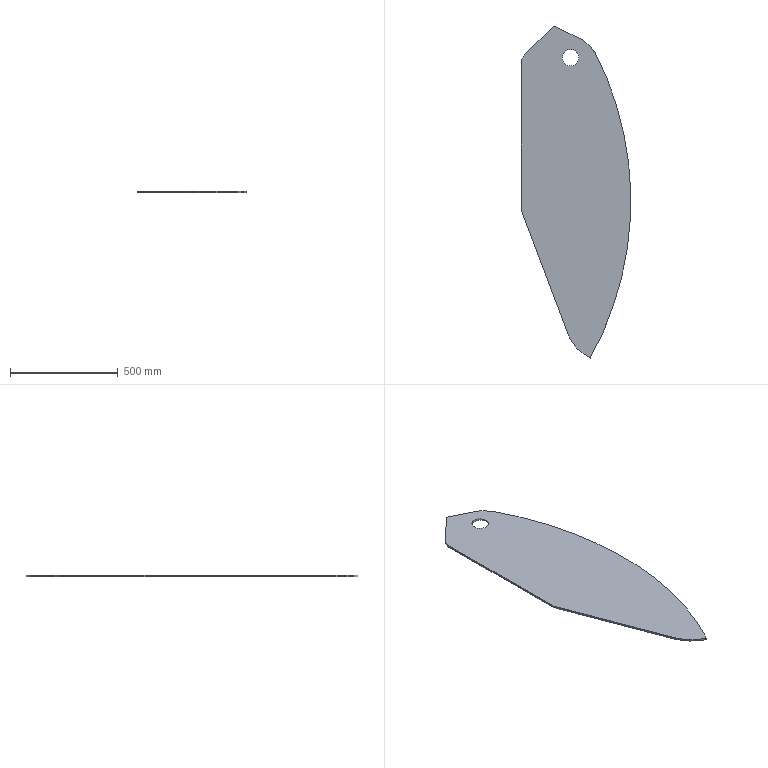Part | SolidWorks | features Extrusion 1 | 1 solid | 13 faces | box 508 x 1540 x 8 mm | volume 4517145 mm3 | plane 7 | cylinder 6 | commonest cylinder face diameters 76.2 x2 101.6 x1 279.4 x1 406.4 x1 3016 x1
STEP:
#1=CARTESIAN_POINT('',(1190.625,663.575,4.));
#2=VERTEX_POINT('',#1);
#3=CARTESIAN_POINT('',(1266.825,663.575,4.));
#4=VERTEX_POINT('',#3);
#5=CARTESIAN_POINT('',(1228.725,663.575,4.));
#6=DIRECTION('',(0.,0.,1.));
#7=DIRECTION('',(1.,0.,0.));
#8=AXIS2_PLACEMENT_3D('',#5,#6,#7);
#9=CIRCLE('',#8,38.1);
#10=EDGE_CURVE('',#2,#4,#9,.T.);
#11=ORIENTED_EDGE('',*,*,#10,.T.);
#12=CARTESIAN_POINT('',(1266.825,663.575,-4.));
#13=VERTEX_POINT('',#12);
#14=CARTESIAN_POINT('',(1266.825,663.575,4.));
#15=DIRECTION('',(0.,0.,-1.));
#16=VECTOR('',#15,1000.);
#17=LINE('',#14,#16);
#18=EDGE_CURVE('',#4,#13,#17,.T.);
#19=ORIENTED_EDGE('',*,*,#18,.T.);
#20=CARTESIAN_POINT('',(1190.625,663.575,-4.));
#21=VERTEX_POINT('',#20);
#22=CARTESIAN_POINT('',(1228.725,663.575,-4.));
#23=DIRECTION('',(0.,0.,1.));
#24=DIRECTION('',(1.,0.,0.));
#25=AXIS2_PLACEMENT_3D('',#22,#23,#24);
#26=CIRCLE('',#25,38.1);
#27=EDGE_CURVE('',#21,#13,#26,.T.);
#28=ORIENTED_EDGE('',*,*,#27,.F.);
#29=CARTESIAN_POINT('',(1190.625,663.575,4.));
#30=DIRECTION('',(0.,0.,-1.));
#31=VECTOR('',#30,1000.);
#32=LINE('',#29,#31);
#33=EDGE_CURVE('',#2,#21,#32,.T.);
#34=ORIENTED_EDGE('',*,*,#33,.F.);
#35=EDGE_LOOP('',(#11,#19,#28,#34));
#36=FACE_OUTER_BOUND('',#35,.T.);
#37=CARTESIAN_POINT('',(1228.725,663.575,4.));
#38=DIRECTION('',(0.,0.,-1.));
#39=DIRECTION('',(-1.,0.,0.));
#40=AXIS2_PLACEMENT_3D('',#37,#38,#39);
#41=CYLINDRICAL_SURFACE('',#40,38.1);
#42=ADVANCED_FACE('',(#36),#41,.F.);
#43=CARTESIAN_POINT('',(1015.696,677.95,4.));
#44=VERTEX_POINT('',#43);
#45=CARTESIAN_POINT('',(1000.125,641.35,4.));
#46=VERTEX_POINT('',#45);
#47=CARTESIAN_POINT('',(1050.925,641.35,4.));
#48=DIRECTION('',(0.,0.,1.));
#49=DIRECTION('',(1.,0.,0.));
#50=AXIS2_PLACEMENT_3D('',#47,#48,#49);
#51=CIRCLE('',#50,50.8);
#52=EDGE_CURVE('',#44,#46,#51,.T.);
#53=ORIENTED_EDGE('',*,*,#52,.T.);
#54=CARTESIAN_POINT('',(1000.125,-45.063,4.));
#55=VERTEX_POINT('',#54);
#56=CARTESIAN_POINT('',(1000.125,641.35,4.));
#57=DIRECTION('',(0.,-1.,0.));
#58=VECTOR('',#57,1000.);
#59=LINE('',#56,#58);
#60=EDGE_CURVE('',#46,#55,#59,.T.);
#61=ORIENTED_EDGE('',*,*,#60,.T.);
#62=CARTESIAN_POINT('',(1215.934,-617.114,4.));
#63=VERTEX_POINT('',#62);
#64=CARTESIAN_POINT('',(1000.125,-45.063,4.));
#65=DIRECTION('',(0.353,-0.9356,0.));
#66=VECTOR('',#65,1000.);
#67=LINE('',#64,#66);
#68=EDGE_CURVE('',#55,#63,#67,.T.);
#69=ORIENTED_EDGE('',*,*,#68,.T.);
#70=CARTESIAN_POINT('',(1319.975,-729.456,4.));
#71=VERTEX_POINT('',#70);
#72=CARTESIAN_POINT('',(1406.055,-545.39,4.));
#73=DIRECTION('',(0.,0.,1.));
#74=DIRECTION('',(1.,0.,0.));
#75=AXIS2_PLACEMENT_3D('',#72,#73,#74);
#76=CIRCLE('',#75,203.2);
#77=EDGE_CURVE('',#63,#71,#76,.T.);
#78=ORIENTED_EDGE('',*,*,#77,.T.);
#79=CARTESIAN_POINT('',(1339.914,692.15,4.));
#80=VERTEX_POINT('',#79);
#81=CARTESIAN_POINT('',(0.,0.,4.));
#82=DIRECTION('',(0.,0.,1.));
#83=DIRECTION('',(1.,0.,0.));
#84=AXIS2_PLACEMENT_3D('',#81,#82,#83);
#85=CIRCLE('',#84,1508.125);
#86=EDGE_CURVE('',#71,#80,#85,.T.);
#87=ORIENTED_EDGE('',*,*,#86,.T.);
#88=CARTESIAN_POINT('',(1336.871,690.572,4.));
#89=VERTEX_POINT('',#88);
#90=CARTESIAN_POINT('',(1339.914,692.15,4.));
#91=DIRECTION('',(-0.8878,-0.4603,0.));
#92=VECTOR('',#91,1000.);
#93=LINE('',#90,#92);
#94=EDGE_CURVE('',#80,#89,#93,.T.);
#95=ORIENTED_EDGE('',*,*,#94,.T.);
#96=CARTESIAN_POINT('',(1273.824,751.96,4.));
#97=VERTEX_POINT('',#96);
#98=CARTESIAN_POINT('',(1212.85,626.269,4.));
#99=DIRECTION('',(0.,0.,1.));
#100=DIRECTION('',(1.,0.,0.));
#101=AXIS2_PLACEMENT_3D('',#98,#99,#100);
#102=CIRCLE('',#101,139.7);
#103=EDGE_CURVE('',#89,#97,#102,.T.);
#104=ORIENTED_EDGE('',*,*,#103,.T.);
#105=CARTESIAN_POINT('',(1153.319,810.419,4.));
#106=VERTEX_POINT('',#105);
#107=CARTESIAN_POINT('',(1153.319,810.419,4.));
#108=DIRECTION('',(-0.8997,0.4365,0.));
#109=VECTOR('',#108,1000.);
#110=LINE('',#107,#109);
#111=EDGE_CURVE('',#97,#106,#110,.T.);
#112=ORIENTED_EDGE('',*,*,#111,.T.);
#113=CARTESIAN_POINT('',(1153.319,810.419,4.));
#114=DIRECTION('',(-0.7205,-0.6935,0.));
#115=VECTOR('',#114,1000.);
#116=LINE('',#113,#115);
#117=EDGE_CURVE('',#106,#44,#116,.T.);
#118=ORIENTED_EDGE('',*,*,#117,.T.);
#119=EDGE_LOOP('',(#53,#61,#69,#78,#87,#95,#104,#112,#118));
#120=FACE_OUTER_BOUND('',#119,.T.);
#121=ORIENTED_EDGE('',*,*,#10,.F.);
#122=CARTESIAN_POINT('',(1228.725,663.575,4.));
#123=DIRECTION('',(0.,0.,1.));
#124=DIRECTION('',(1.,0.,0.));
#125=AXIS2_PLACEMENT_3D('',#122,#123,#124);
#126=CIRCLE('',#125,38.1);
#127=EDGE_CURVE('',#4,#2,#126,.T.);
#128=ORIENTED_EDGE('',*,*,#127,.F.);
#129=EDGE_LOOP('',(#121,#128));
#130=FACE_BOUND('',#129,.T.);
#131=CARTESIAN_POINT('',(1050.925,641.35,4.));
#132=DIRECTION('',(0.,0.,1.));
#133=DIRECTION('',(1.,0.,0.));
#134=AXIS2_PLACEMENT_3D('',#131,#132,#133);
#135=PLANE('',#134);
#136=ADVANCED_FACE('',(#120,#130),#135,.T.);
#137=CARTESIAN_POINT('',(1015.696,677.95,-4.));
#138=VERTEX_POINT('',#137);
#139=CARTESIAN_POINT('',(1000.125,641.35,-4.));
#140=VERTEX_POINT('',#139);
#141=CARTESIAN_POINT('',(1050.925,641.35,-4.));
#142=DIRECTION('',(0.,0.,1.));
#143=DIRECTION('',(1.,0.,0.));
#144=AXIS2_PLACEMENT_3D('',#141,#142,#143);
#145=CIRCLE('',#144,50.8);
#146=EDGE_CURVE('',#138,#140,#145,.T.);
#147=ORIENTED_EDGE('',*,*,#146,.F.);
#148=CARTESIAN_POINT('',(1153.319,810.419,-4.));
#149=VERTEX_POINT('',#148);
#150=CARTESIAN_POINT('',(1153.319,810.419,-4.));
#151=DIRECTION('',(-0.7205,-0.6935,0.));
#152=VECTOR('',#151,1000.);
#153=LINE('',#150,#152);
#154=EDGE_CURVE('',#149,#138,#153,.T.);
#155=ORIENTED_EDGE('',*,*,#154,.F.);
#156=CARTESIAN_POINT('',(1273.824,751.96,-4.));
#157=VERTEX_POINT('',#156);
#158=CARTESIAN_POINT('',(1153.319,810.419,-4.));
#159=DIRECTION('',(-0.8997,0.4365,0.));
#160=VECTOR('',#159,1000.);
#161=LINE('',#158,#160);
#162=EDGE_CURVE('',#157,#149,#161,.T.);
#163=ORIENTED_EDGE('',*,*,#162,.F.);
#164=CARTESIAN_POINT('',(1336.871,690.572,-4.));
#165=VERTEX_POINT('',#164);
#166=CARTESIAN_POINT('',(1212.85,626.269,-4.));
#167=DIRECTION('',(0.,0.,1.));
#168=DIRECTION('',(1.,0.,0.));
#169=AXIS2_PLACEMENT_3D('',#166,#167,#168);
#170=CIRCLE('',#169,139.7);
#171=EDGE_CURVE('',#165,#157,#170,.T.);
#172=ORIENTED_EDGE('',*,*,#171,.F.);
#173=CARTESIAN_POINT('',(1339.914,692.15,-4.));
#174=VERTEX_POINT('',#173);
#175=CARTESIAN_POINT('',(1339.914,692.15,-4.));
#176=DIRECTION('',(-0.8878,-0.4603,0.));
#177=VECTOR('',#176,1000.);
#178=LINE('',#175,#177);
#179=EDGE_CURVE('',#174,#165,#178,.T.);
#180=ORIENTED_EDGE('',*,*,#179,.F.);
#181=CARTESIAN_POINT('',(1319.975,-729.456,-4.));
#182=VERTEX_POINT('',#181);
#183=CARTESIAN_POINT('',(0.,0.,-4.));
#184=DIRECTION('',(0.,0.,1.));
#185=DIRECTION('',(1.,0.,0.));
#186=AXIS2_PLACEMENT_3D('',#183,#184,#185);
#187=CIRCLE('',#186,1508.125);
#188=EDGE_CURVE('',#182,#174,#187,.T.);
#189=ORIENTED_EDGE('',*,*,#188,.F.);
#190=CARTESIAN_POINT('',(1215.934,-617.114,-4.));
#191=VERTEX_POINT('',#190);
#192=CARTESIAN_POINT('',(1406.055,-545.39,-4.));
#193=DIRECTION('',(0.,0.,1.));
#194=DIRECTION('',(1.,0.,0.));
#195=AXIS2_PLACEMENT_3D('',#192,#193,#194);
#196=CIRCLE('',#195,203.2);
#197=EDGE_CURVE('',#191,#182,#196,.T.);
#198=ORIENTED_EDGE('',*,*,#197,.F.);
#199=CARTESIAN_POINT('',(1000.125,-45.063,-4.));
#200=VERTEX_POINT('',#199);
#201=CARTESIAN_POINT('',(1000.125,-45.063,-4.));
#202=DIRECTION('',(0.353,-0.9356,0.));
#203=VECTOR('',#202,1000.);
#204=LINE('',#201,#203);
#205=EDGE_CURVE('',#200,#191,#204,.T.);
#206=ORIENTED_EDGE('',*,*,#205,.F.);
#207=CARTESIAN_POINT('',(1000.125,641.35,-4.));
#208=DIRECTION('',(0.,-1.,0.));
#209=VECTOR('',#208,1000.);
#210=LINE('',#207,#209);
#211=EDGE_CURVE('',#140,#200,#210,.T.);
#212=ORIENTED_EDGE('',*,*,#211,.F.);
#213=EDGE_LOOP('',(#147,#155,#163,#172,#180,#189,#198,#206,#212));
#214=FACE_OUTER_BOUND('',#213,.T.);
#215=ORIENTED_EDGE('',*,*,#27,.T.);
#216=CARTESIAN_POINT('',(1228.725,663.575,-4.));
#217=DIRECTION('',(0.,0.,1.));
#218=DIRECTION('',(1.,0.,0.));
#219=AXIS2_PLACEMENT_3D('',#216,#217,#218);
#220=CIRCLE('',#219,38.1);
#221=EDGE_CURVE('',#13,#21,#220,.T.);
#222=ORIENTED_EDGE('',*,*,#221,.T.);
#223=EDGE_LOOP('',(#215,#222));
#224=FACE_BOUND('',#223,.T.);
#225=CARTESIAN_POINT('',(1050.925,641.35,-4.));
#226=DIRECTION('',(0.,0.,1.));
#227=DIRECTION('',(1.,0.,0.));
#228=AXIS2_PLACEMENT_3D('',#225,#226,#227);
#229=PLANE('',#228);
#230=ADVANCED_FACE('',(#214,#224),#229,.F.);
#231=ORIENTED_EDGE('',*,*,#146,.T.);
#232=CARTESIAN_POINT('',(1000.125,641.35,4.));
#233=DIRECTION('',(0.,0.,-1.));
#234=VECTOR('',#233,1000.);
#235=LINE('',#232,#234);
#236=EDGE_CURVE('',#46,#140,#235,.T.);
#237=ORIENTED_EDGE('',*,*,#236,.F.);
#238=ORIENTED_EDGE('',*,*,#52,.F.);
#239=CARTESIAN_POINT('',(1015.696,677.95,4.));
#240=DIRECTION('',(0.,0.,-1.));
#241=VECTOR('',#240,1000.);
#242=LINE('',#239,#241);
#243=EDGE_CURVE('',#44,#138,#242,.T.);
#244=ORIENTED_EDGE('',*,*,#243,.T.);
#245=EDGE_LOOP('',(#231,#237,#238,#244));
#246=FACE_OUTER_BOUND('',#245,.T.);
#247=CARTESIAN_POINT('',(1050.925,641.35,4.));
#248=DIRECTION('',(0.,0.,-1.));
#249=DIRECTION('',(-1.,0.,0.));
#250=AXIS2_PLACEMENT_3D('',#247,#248,#249);
#251=CYLINDRICAL_SURFACE('',#250,50.8);
#252=ADVANCED_FACE('',(#246),#251,.T.);
#253=ORIENTED_EDGE('',*,*,#211,.T.);
#254=CARTESIAN_POINT('',(1000.125,-45.063,4.));
#255=DIRECTION('',(0.,0.,-1.));
#256=VECTOR('',#255,1000.);
#257=LINE('',#254,#256);
#258=EDGE_CURVE('',#55,#200,#257,.T.);
#259=ORIENTED_EDGE('',*,*,#258,.F.);
#260=ORIENTED_EDGE('',*,*,#60,.F.);
#261=ORIENTED_EDGE('',*,*,#236,.T.);
#262=EDGE_LOOP('',(#253,#259,#260,#261));
#263=FACE_OUTER_BOUND('',#262,.T.);
#264=CARTESIAN_POINT('',(1000.125,641.35,4.));
#265=DIRECTION('',(1.,0.,0.));
#266=DIRECTION('',(0.,1.,0.));
#267=AXIS2_PLACEMENT_3D('',#264,#265,#266);
#268=PLANE('',#267);
#269=ADVANCED_FACE('',(#263),#268,.F.);
#270=ORIENTED_EDGE('',*,*,#205,.T.);
#271=CARTESIAN_POINT('',(1215.934,-617.114,4.));
#272=DIRECTION('',(0.,0.,-1.));
#273=VECTOR('',#272,1000.);
#274=LINE('',#271,#273);
#275=EDGE_CURVE('',#63,#191,#274,.T.);
#276=ORIENTED_EDGE('',*,*,#275,.F.);
#277=ORIENTED_EDGE('',*,*,#68,.F.);
#278=ORIENTED_EDGE('',*,*,#258,.T.);
#279=EDGE_LOOP('',(#270,#276,#277,#278));
#280=FACE_OUTER_BOUND('',#279,.T.);
#281=CARTESIAN_POINT('',(1000.125,-45.063,4.));
#282=DIRECTION('',(0.9356,0.353,0.));
#283=DIRECTION('',(-0.353,0.9356,0.));
#284=AXIS2_PLACEMENT_3D('',#281,#282,#283);
#285=PLANE('',#284);
#286=ADVANCED_FACE('',(#280),#285,.F.);
#287=ORIENTED_EDGE('',*,*,#197,.T.);
#288=CARTESIAN_POINT('',(1319.975,-729.456,4.));
#289=DIRECTION('',(0.,0.,-1.));
#290=VECTOR('',#289,1000.);
#291=LINE('',#288,#290);
#292=EDGE_CURVE('',#71,#182,#291,.T.);
#293=ORIENTED_EDGE('',*,*,#292,.F.);
#294=ORIENTED_EDGE('',*,*,#77,.F.);
#295=ORIENTED_EDGE('',*,*,#275,.T.);
#296=EDGE_LOOP('',(#287,#293,#294,#295));
#297=FACE_OUTER_BOUND('',#296,.T.);
#298=CARTESIAN_POINT('',(1406.055,-545.39,4.));
#299=DIRECTION('',(0.,0.,-1.));
#300=DIRECTION('',(-1.,0.,0.));
#301=AXIS2_PLACEMENT_3D('',#298,#299,#300);
#302=CYLINDRICAL_SURFACE('',#301,203.2);
#303=ADVANCED_FACE('',(#297),#302,.T.);
#304=ORIENTED_EDGE('',*,*,#188,.T.);
#305=CARTESIAN_POINT('',(1339.914,692.15,4.));
#306=DIRECTION('',(0.,0.,-1.));
#307=VECTOR('',#306,1000.);
#308=LINE('',#305,#307);
#309=EDGE_CURVE('',#80,#174,#308,.T.);
#310=ORIENTED_EDGE('',*,*,#309,.F.);
#311=ORIENTED_EDGE('',*,*,#86,.F.);
#312=ORIENTED_EDGE('',*,*,#292,.T.);
#313=EDGE_LOOP('',(#304,#310,#311,#312));
#314=FACE_OUTER_BOUND('',#313,.T.);
#315=CARTESIAN_POINT('',(0.,0.,4.));
#316=DIRECTION('',(0.,0.,-1.));
#317=DIRECTION('',(-1.,0.,0.));
#318=AXIS2_PLACEMENT_3D('',#315,#316,#317);
#319=CYLINDRICAL_SURFACE('',#318,1508.125);
#320=ADVANCED_FACE('',(#314),#319,.T.);
#321=ORIENTED_EDGE('',*,*,#179,.T.);
#322=CARTESIAN_POINT('',(1336.871,690.572,4.));
#323=DIRECTION('',(0.,0.,-1.));
#324=VECTOR('',#323,1000.);
#325=LINE('',#322,#324);
#326=EDGE_CURVE('',#89,#165,#325,.T.);
#327=ORIENTED_EDGE('',*,*,#326,.F.);
#328=ORIENTED_EDGE('',*,*,#94,.F.);
#329=ORIENTED_EDGE('',*,*,#309,.T.);
#330=EDGE_LOOP('',(#321,#327,#328,#329));
#331=FACE_OUTER_BOUND('',#330,.T.);
#332=CARTESIAN_POINT('',(1339.914,692.15,4.));
#333=DIRECTION('',(0.4603,-0.8878,0.));
#334=DIRECTION('',(0.8878,0.4603,0.));
#335=AXIS2_PLACEMENT_3D('',#332,#333,#334);
#336=PLANE('',#335);
#337=ADVANCED_FACE('',(#331),#336,.F.);
#338=ORIENTED_EDGE('',*,*,#171,.T.);
#339=CARTESIAN_POINT('',(1273.824,751.96,4.));
#340=DIRECTION('',(0.,0.,-1.));
#341=VECTOR('',#340,1000.);
#342=LINE('',#339,#341);
#343=EDGE_CURVE('',#97,#157,#342,.T.);
#344=ORIENTED_EDGE('',*,*,#343,.F.);
#345=ORIENTED_EDGE('',*,*,#103,.F.);
#346=ORIENTED_EDGE('',*,*,#326,.T.);
#347=EDGE_LOOP('',(#338,#344,#345,#346));
#348=FACE_OUTER_BOUND('',#347,.T.);
#349=CARTESIAN_POINT('',(1212.85,626.269,4.));
#350=DIRECTION('',(0.,0.,-1.));
#351=DIRECTION('',(-1.,0.,0.));
#352=AXIS2_PLACEMENT_3D('',#349,#350,#351);
#353=CYLINDRICAL_SURFACE('',#352,139.7);
#354=ADVANCED_FACE('',(#348),#353,.T.);
#355=ORIENTED_EDGE('',*,*,#162,.T.);
#356=CARTESIAN_POINT('',(1153.319,810.419,4.));
#357=DIRECTION('',(0.,0.,-1.));
#358=VECTOR('',#357,1000.);
#359=LINE('',#356,#358);
#360=EDGE_CURVE('',#106,#149,#359,.T.);
#361=ORIENTED_EDGE('',*,*,#360,.F.);
#362=ORIENTED_EDGE('',*,*,#111,.F.);
#363=ORIENTED_EDGE('',*,*,#343,.T.);
#364=EDGE_LOOP('',(#355,#361,#362,#363));
#365=FACE_OUTER_BOUND('',#364,.T.);
#366=CARTESIAN_POINT('',(1153.319,810.419,4.));
#367=DIRECTION('',(-0.4365,-0.8997,0.));
#368=DIRECTION('',(0.8997,-0.4365,0.));
#369=AXIS2_PLACEMENT_3D('',#366,#367,#368);
#370=PLANE('',#369);
#371=ADVANCED_FACE('',(#365),#370,.F.);
#372=ORIENTED_EDGE('',*,*,#154,.T.);
#373=ORIENTED_EDGE('',*,*,#243,.F.);
#374=ORIENTED_EDGE('',*,*,#117,.F.);
#375=ORIENTED_EDGE('',*,*,#360,.T.);
#376=EDGE_LOOP('',(#372,#373,#374,#375));
#377=FACE_OUTER_BOUND('',#376,.T.);
#378=CARTESIAN_POINT('',(1153.319,810.419,4.));
#379=DIRECTION('',(0.6935,-0.7205,0.));
#380=DIRECTION('',(0.7205,0.6935,0.));
#381=AXIS2_PLACEMENT_3D('',#378,#379,#380);
#382=PLANE('',#381);
#383=ADVANCED_FACE('',(#377),#382,.F.);
#384=ORIENTED_EDGE('',*,*,#18,.F.);
#385=ORIENTED_EDGE('',*,*,#127,.T.);
#386=ORIENTED_EDGE('',*,*,#33,.T.);
#387=ORIENTED_EDGE('',*,*,#221,.F.);
#388=EDGE_LOOP('',(#384,#385,#386,#387));
#389=FACE_OUTER_BOUND('',#388,.T.);
#390=CARTESIAN_POINT('',(1228.725,663.575,4.));
#391=DIRECTION('',(0.,0.,-1.));
#392=DIRECTION('',(-1.,0.,0.));
#393=AXIS2_PLACEMENT_3D('',#390,#391,#392);
#394=CYLINDRICAL_SURFACE('',#393,38.1);
#395=ADVANCED_FACE('',(#389),#394,.F.);
#396=CLOSED_SHELL('',(#42,#136,#230,#252,#269,#286,#303,#320,#337,#354,#371,#383,#395));
#397=MANIFOLD_SOLID_BREP('',#396);
#398=CARTESIAN_POINT('',(0.,0.,0.));
#399=DIRECTION('',(0.,0.,1.));
#400=DIRECTION('',(1.,0.,0.));
#401=AXIS2_PLACEMENT_3D('',#398,#399,#400);
#402=(LENGTH_UNIT()NAMED_UNIT(*)SI_UNIT(.MILLI.,.METRE.));
#403=UNCERTAINTY_MEASURE_WITH_UNIT(LENGTH_MEASURE(0.00001),#402,'','');
#404=(NAMED_UNIT(*)PLANE_ANGLE_UNIT()SI_UNIT($,.RADIAN.));
#405=(NAMED_UNIT(*)SI_UNIT($,.STERADIAN.)SOLID_ANGLE_UNIT());
#406=(GEOMETRIC_REPRESENTATION_CONTEXT(3)GLOBAL_UNCERTAINTY_ASSIGNED_CONTEXT((#403))GLOBAL_UNIT_ASSIGNED_CONTEXT((#402,#404,#405))REPRESENTATION_CONTEXT('',''));
#407=ADVANCED_BREP_SHAPE_REPRESENTATION('',(#397,#401),#406);